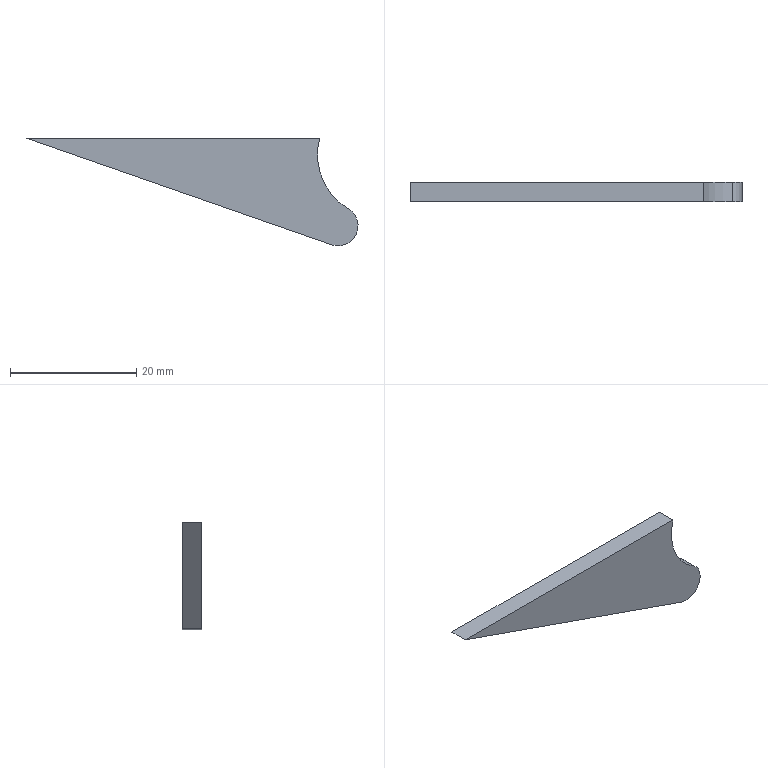Part | NX | features BREP 1 | 1 solid | 6 faces | box 52.551 x 3.023 x 17.042 mm | volume 1259 mm3 | plane 4 | cylinder 2 | commonest cylinder face diameters 6.296 x1 20.015 x1
STEP:
#1=CARTESIAN_POINT('',(46.468,0.,0.));
#2=VERTEX_POINT('',#1);
#3=CARTESIAN_POINT('',(51.014,0.,-11.189));
#4=VERTEX_POINT('',#3);
#5=CARTESIAN_POINT('',(56.134,0.,-2.591));
#6=DIRECTION('',(0.,-1.,0.));
#7=DIRECTION('',(-0.9659,0.,0.2589));
#8=AXIS2_PLACEMENT_3D('',#5,#6,#7);
#9=CIRCLE('',#8,10.008);
#10=EDGE_CURVE('',#2,#4,#9,.T.);
#11=ORIENTED_EDGE('',*,*,#10,.T.);
#12=CARTESIAN_POINT('',(48.367,0.,-16.866));
#13=VERTEX_POINT('',#12);
#14=CARTESIAN_POINT('',(49.403,0.,-13.894));
#15=DIRECTION('',(0.,1.,0.));
#16=DIRECTION('',(0.5117,0.,0.8592));
#17=AXIS2_PLACEMENT_3D('',#14,#15,#16);
#18=CIRCLE('',#17,3.148);
#19=EDGE_CURVE('',#4,#13,#18,.T.);
#20=ORIENTED_EDGE('',*,*,#19,.T.);
#21=CARTESIAN_POINT('',(0.,0.,0.));
#22=VERTEX_POINT('',#21);
#23=CARTESIAN_POINT('',(48.367,0.,-16.866));
#24=DIRECTION('',(-0.9442,0.,0.3293));
#25=VECTOR('',#24,1000.);
#26=LINE('',#23,#25);
#27=EDGE_CURVE('',#13,#22,#26,.T.);
#28=ORIENTED_EDGE('',*,*,#27,.T.);
#29=CARTESIAN_POINT('',(0.,0.,0.));
#30=DIRECTION('',(1.,0.,0.));
#31=VECTOR('',#30,1000.);
#32=LINE('',#29,#31);
#33=EDGE_CURVE('',#22,#2,#32,.T.);
#34=ORIENTED_EDGE('',*,*,#33,.T.);
#35=EDGE_LOOP('',(#11,#20,#28,#34));
#36=FACE_BOUND('',#35,.T.);
#37=CARTESIAN_POINT('',(0.,0.,0.));
#38=DIRECTION('',(0.,1.,0.));
#39=DIRECTION('',(1.,0.,0.));
#40=AXIS2_PLACEMENT_3D('',#37,#38,#39);
#41=PLANE('',#40);
#42=ADVANCED_FACE('',(#36),#41,.T.);
#43=CARTESIAN_POINT('',(0.,-3.023,0.));
#44=VERTEX_POINT('',#43);
#45=CARTESIAN_POINT('',(0.,0.,0.));
#46=DIRECTION('',(0.,-1.,0.));
#47=VECTOR('',#46,1000.);
#48=LINE('',#45,#47);
#49=EDGE_CURVE('',#22,#44,#48,.T.);
#50=ORIENTED_EDGE('',*,*,#49,.T.);
#51=CARTESIAN_POINT('',(46.468,-3.023,0.));
#52=VERTEX_POINT('',#51);
#53=CARTESIAN_POINT('',(0.,-3.023,0.));
#54=DIRECTION('',(1.,0.,0.));
#55=VECTOR('',#54,1000.);
#56=LINE('',#53,#55);
#57=EDGE_CURVE('',#44,#52,#56,.T.);
#58=ORIENTED_EDGE('',*,*,#57,.T.);
#59=CARTESIAN_POINT('',(46.468,0.,0.));
#60=DIRECTION('',(0.,-1.,0.));
#61=VECTOR('',#60,1000.);
#62=LINE('',#59,#61);
#63=EDGE_CURVE('',#2,#52,#62,.T.);
#64=ORIENTED_EDGE('',*,*,#63,.F.);
#65=ORIENTED_EDGE('',*,*,#33,.F.);
#66=EDGE_LOOP('',(#50,#58,#64,#65));
#67=FACE_BOUND('',#66,.T.);
#68=CARTESIAN_POINT('',(23.234,-1.511,0.));
#69=DIRECTION('',(0.,0.,1.));
#70=DIRECTION('',(1.,0.,0.));
#71=AXIS2_PLACEMENT_3D('',#68,#69,#70);
#72=PLANE('',#71);
#73=ADVANCED_FACE('',(#67),#72,.T.);
#74=ORIENTED_EDGE('',*,*,#63,.T.);
#75=CARTESIAN_POINT('',(51.014,-3.023,-11.189));
#76=VERTEX_POINT('',#75);
#77=CARTESIAN_POINT('',(56.134,-3.023,-2.591));
#78=DIRECTION('',(0.,-1.,0.));
#79=DIRECTION('',(-0.9659,0.,0.2589));
#80=AXIS2_PLACEMENT_3D('',#77,#78,#79);
#81=CIRCLE('',#80,10.008);
#82=EDGE_CURVE('',#52,#76,#81,.T.);
#83=ORIENTED_EDGE('',*,*,#82,.T.);
#84=CARTESIAN_POINT('',(51.014,0.,-11.189));
#85=DIRECTION('',(0.,-1.,0.));
#86=VECTOR('',#85,1000.);
#87=LINE('',#84,#86);
#88=EDGE_CURVE('',#4,#76,#87,.T.);
#89=ORIENTED_EDGE('',*,*,#88,.F.);
#90=ORIENTED_EDGE('',*,*,#10,.F.);
#91=EDGE_LOOP('',(#74,#83,#89,#90));
#92=FACE_BOUND('',#91,.T.);
#93=CARTESIAN_POINT('',(56.134,-1.511,-2.591));
#94=DIRECTION('',(0.,-1.,0.));
#95=DIRECTION('',(-0.9659,0.,0.2589));
#96=AXIS2_PLACEMENT_3D('',#93,#94,#95);
#97=CYLINDRICAL_SURFACE('',#96,10.008);
#98=ADVANCED_FACE('',(#92),#97,.F.);
#99=ORIENTED_EDGE('',*,*,#88,.T.);
#100=CARTESIAN_POINT('',(48.367,-3.023,-16.866));
#101=VERTEX_POINT('',#100);
#102=CARTESIAN_POINT('',(49.403,-3.023,-13.894));
#103=DIRECTION('',(0.,1.,0.));
#104=DIRECTION('',(0.5117,0.,0.8592));
#105=AXIS2_PLACEMENT_3D('',#102,#103,#104);
#106=CIRCLE('',#105,3.148);
#107=EDGE_CURVE('',#76,#101,#106,.T.);
#108=ORIENTED_EDGE('',*,*,#107,.T.);
#109=CARTESIAN_POINT('',(48.367,0.,-16.866));
#110=DIRECTION('',(0.,-1.,0.));
#111=VECTOR('',#110,1000.);
#112=LINE('',#109,#111);
#113=EDGE_CURVE('',#13,#101,#112,.T.);
#114=ORIENTED_EDGE('',*,*,#113,.F.);
#115=ORIENTED_EDGE('',*,*,#19,.F.);
#116=EDGE_LOOP('',(#99,#108,#114,#115));
#117=FACE_BOUND('',#116,.T.);
#118=CARTESIAN_POINT('',(49.403,-1.511,-13.894));
#119=DIRECTION('',(0.,1.,0.));
#120=DIRECTION('',(0.5117,0.,0.8592));
#121=AXIS2_PLACEMENT_3D('',#118,#119,#120);
#122=CYLINDRICAL_SURFACE('',#121,3.148);
#123=ADVANCED_FACE('',(#117),#122,.T.);
#124=ORIENTED_EDGE('',*,*,#113,.T.);
#125=CARTESIAN_POINT('',(48.367,-3.023,-16.866));
#126=DIRECTION('',(-0.9442,0.,0.3293));
#127=VECTOR('',#126,1000.);
#128=LINE('',#125,#127);
#129=EDGE_CURVE('',#101,#44,#128,.T.);
#130=ORIENTED_EDGE('',*,*,#129,.T.);
#131=ORIENTED_EDGE('',*,*,#49,.F.);
#132=ORIENTED_EDGE('',*,*,#27,.F.);
#133=EDGE_LOOP('',(#124,#130,#131,#132));
#134=FACE_BOUND('',#133,.T.);
#135=CARTESIAN_POINT('',(24.183,-1.511,-8.433));
#136=DIRECTION('',(-0.3293,0.,-0.9442));
#137=DIRECTION('',(-0.9442,0.,0.3293));
#138=AXIS2_PLACEMENT_3D('',#135,#136,#137);
#139=PLANE('',#138);
#140=ADVANCED_FACE('',(#134),#139,.T.);
#141=ORIENTED_EDGE('',*,*,#129,.F.);
#142=ORIENTED_EDGE('',*,*,#107,.F.);
#143=ORIENTED_EDGE('',*,*,#82,.F.);
#144=ORIENTED_EDGE('',*,*,#57,.F.);
#145=EDGE_LOOP('',(#141,#142,#143,#144));
#146=FACE_BOUND('',#145,.T.);
#147=CARTESIAN_POINT('',(0.,-3.023,0.));
#148=DIRECTION('',(0.,1.,0.));
#149=DIRECTION('',(1.,0.,0.));
#150=AXIS2_PLACEMENT_3D('',#147,#148,#149);
#151=PLANE('',#150);
#152=ADVANCED_FACE('',(#146),#151,.F.);
#153=CLOSED_SHELL('',(#42,#73,#98,#123,#140,#152));
#154=MANIFOLD_SOLID_BREP('',#153);
#155=(LENGTH_UNIT()NAMED_UNIT(*)SI_UNIT(.MILLI.,.METRE.));
#156=UNCERTAINTY_MEASURE_WITH_UNIT(LENGTH_MEASURE(0.00001),#155,'','');
#157=(NAMED_UNIT(*)PLANE_ANGLE_UNIT()SI_UNIT($,.RADIAN.));
#158=(NAMED_UNIT(*)SI_UNIT($,.STERADIAN.)SOLID_ANGLE_UNIT());
#159=(GEOMETRIC_REPRESENTATION_CONTEXT(3)GLOBAL_UNCERTAINTY_ASSIGNED_CONTEXT((#156))GLOBAL_UNIT_ASSIGNED_CONTEXT((#155,#157,#158))REPRESENTATION_CONTEXT('',''));
#160=ADVANCED_BREP_SHAPE_REPRESENTATION('',(#154),#159);